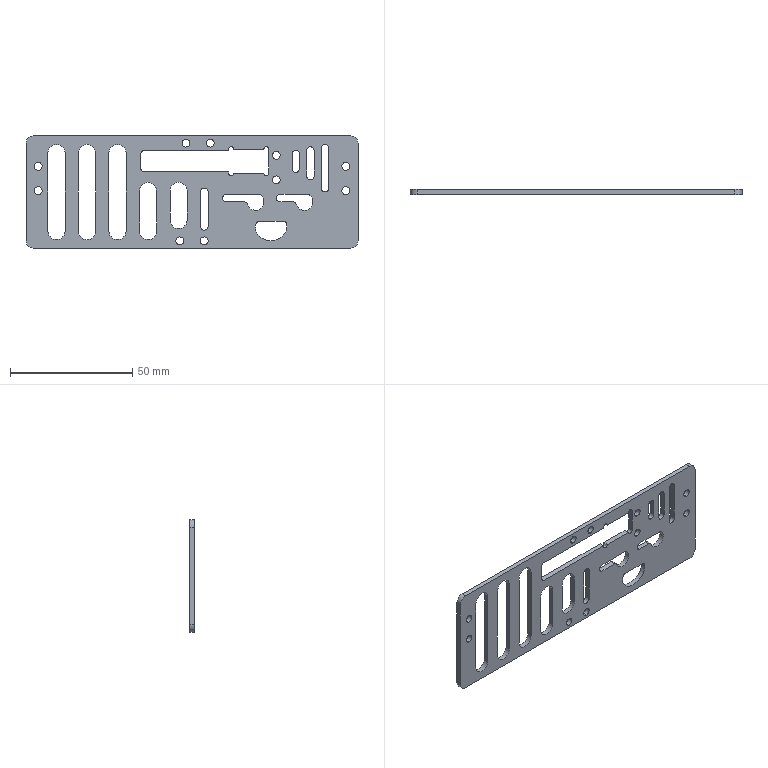Part | SolidWorks | features Fillet 2, Extrusion 1, ICE 1 | 1 solid | 108 faces | box 136 x 2 x 46 mm | volume 8461 mm3 | cylinder 69 | plane 37 | spline 2 | commonest cylinder face diameters 3.2 x23 3 x19 7 x17 2.1 x6 6 x4